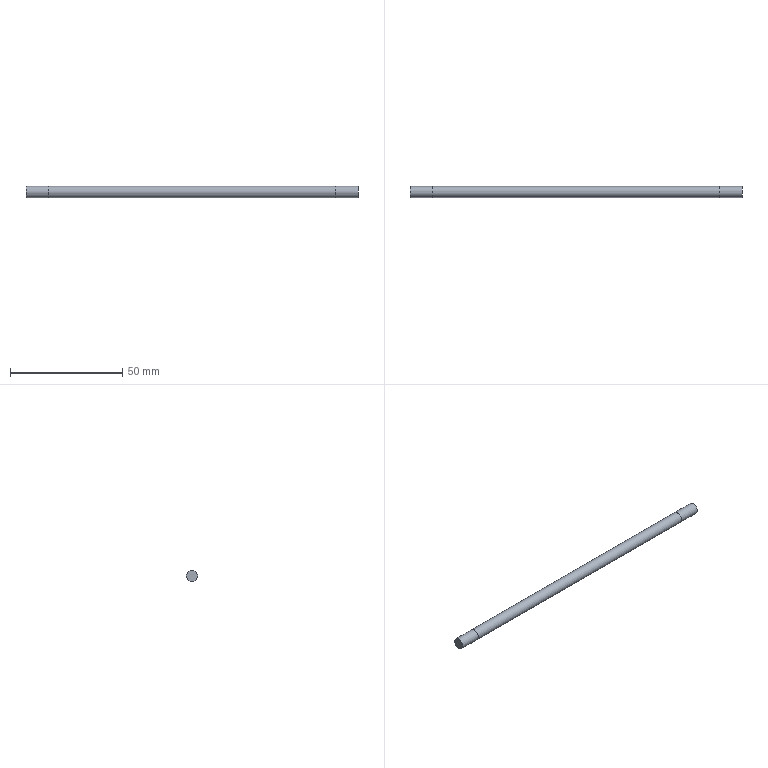Part | STEP file | 1-69.9 | 1 solid | 5 faces | box 148 x 5 x 5 mm | volume 2906 mm3 | cylinder 3 | plane 2 | commonest cylinder face diameters 5 x3
STEP:
#1=CARTESIAN_POINT('',(0.,0.,0.));
#2=DIRECTION('',(0.,0.,1.));
#3=DIRECTION('',(1.,0.,0.));
#4=AXIS2_PLACEMENT_3D('',#1,#2,#3);
#5=CARTESIAN_POINT('',(74.,2.5,0.));
#6=VERTEX_POINT('',#5);
#7=CARTESIAN_POINT('',(74.,0.,0.));
#8=DIRECTION('',(1.,0.,0.));
#9=DIRECTION('',(0.,1.,0.));
#10=AXIS2_PLACEMENT_3D('',#7,#8,#9);
#11=CIRCLE('',#10,2.5);
#12=CARTESIAN_POINT('',(74.,-0.6699,0.));
#13=DIRECTION('',(1.,0.,0.));
#14=DIRECTION('',(0.,1.,0.));
#15=AXIS2_PLACEMENT_3D('',#12,#13,#14);
#16=PLANE('',#15);
#17=CARTESIAN_POINT('',(0.6699,0.));
#18=DIRECTION('',(1.,0.));
#19=AXIS2_PLACEMENT_2D('',#17,#18);
#20=CIRCLE('',#19,2.5);
#21=(GEOMETRIC_REPRESENTATION_CONTEXT(2)PARAMETRIC_REPRESENTATION_CONTEXT()REPRESENTATION_CONTEXT('',''));
#22=DEFINITIONAL_REPRESENTATION('',(#20),#21);
#23=PCURVE('',#16,#22);
#24=CARTESIAN_POINT('',(74.,0.,0.));
#25=DIRECTION('',(-1.,0.,0.));
#26=DIRECTION('',(0.,1.,0.));
#27=AXIS2_PLACEMENT_3D('',#24,#25,#26);
#28=CYLINDRICAL_SURFACE('',#27,2.5);
#29=CARTESIAN_POINT('',(6.283,0.));
#30=DIRECTION('',(-1.,0.));
#31=VECTOR('',#30,1.);
#32=LINE('',#29,#31);
#33=(GEOMETRIC_REPRESENTATION_CONTEXT(2)PARAMETRIC_REPRESENTATION_CONTEXT()REPRESENTATION_CONTEXT('',''));
#34=DEFINITIONAL_REPRESENTATION('',(#32),#33);
#35=PCURVE('',#28,#34);
#36=SURFACE_CURVE('',#11,(#23,#35),.PCURVE_S1.);
#37=EDGE_CURVE('',#6,#6,#36,.T.);
#38=ORIENTED_EDGE('',*,*,#37,.T.);
#39=EDGE_LOOP('',(#38));
#40=FACE_BOUND('',#39,.T.);
#41=ADVANCED_FACE('',(#40),#16,.T.);
#42=CARTESIAN_POINT('',(-74.,2.5,0.));
#43=VERTEX_POINT('',#42);
#44=CARTESIAN_POINT('',(-74.,0.,0.));
#45=DIRECTION('',(1.,0.,0.));
#46=DIRECTION('',(0.,1.,0.));
#47=AXIS2_PLACEMENT_3D('',#44,#45,#46);
#48=CIRCLE('',#47,2.5);
#49=CARTESIAN_POINT('',(-74.,-0.6699,0.));
#50=DIRECTION('',(1.,0.,0.));
#51=DIRECTION('',(0.,1.,0.));
#52=AXIS2_PLACEMENT_3D('',#49,#50,#51);
#53=PLANE('',#52);
#54=CARTESIAN_POINT('',(0.6699,0.));
#55=DIRECTION('',(1.,0.));
#56=AXIS2_PLACEMENT_2D('',#54,#55);
#57=CIRCLE('',#56,2.5);
#58=(GEOMETRIC_REPRESENTATION_CONTEXT(2)PARAMETRIC_REPRESENTATION_CONTEXT()REPRESENTATION_CONTEXT('',''));
#59=DEFINITIONAL_REPRESENTATION('',(#57),#58);
#60=PCURVE('',#53,#59);
#61=CARTESIAN_POINT('',(-64.,0.,0.));
#62=DIRECTION('',(-1.,0.,0.));
#63=DIRECTION('',(0.,1.,0.));
#64=AXIS2_PLACEMENT_3D('',#61,#62,#63);
#65=CYLINDRICAL_SURFACE('',#64,2.5);
#66=CARTESIAN_POINT('',(6.283,10.));
#67=DIRECTION('',(-1.,0.));
#68=VECTOR('',#67,1.);
#69=LINE('',#66,#68);
#70=(GEOMETRIC_REPRESENTATION_CONTEXT(2)PARAMETRIC_REPRESENTATION_CONTEXT()REPRESENTATION_CONTEXT('',''));
#71=DEFINITIONAL_REPRESENTATION('',(#69),#70);
#72=PCURVE('',#65,#71);
#73=SURFACE_CURVE('',#48,(#60,#72),.PCURVE_S1.);
#74=EDGE_CURVE('',#43,#43,#73,.T.);
#75=ORIENTED_EDGE('',*,*,#74,.T.);
#76=EDGE_LOOP('',(#75));
#77=FACE_BOUND('',#76,.F.);
#78=ADVANCED_FACE('',(#77),#53,.F.);
#79=CARTESIAN_POINT('',(64.,2.5,0.));
#80=VERTEX_POINT('',#79);
#81=CARTESIAN_POINT('',(74.,2.5,0.));
#82=DIRECTION('',(-1.,0.,0.));
#83=VECTOR('',#82,1.);
#84=LINE('',#81,#83);
#85=CARTESIAN_POINT('',(6.283,0.));
#86=DIRECTION('',(0.,1.));
#87=VECTOR('',#86,1.);
#88=LINE('',#85,#87);
#89=(GEOMETRIC_REPRESENTATION_CONTEXT(2)PARAMETRIC_REPRESENTATION_CONTEXT()REPRESENTATION_CONTEXT('',''));
#90=DEFINITIONAL_REPRESENTATION('',(#88),#89);
#91=PCURVE('',#28,#90);
#92=CARTESIAN_POINT('',(0.,0.));
#93=DIRECTION('',(0.,1.));
#94=VECTOR('',#93,1.);
#95=LINE('',#92,#94);
#96=(GEOMETRIC_REPRESENTATION_CONTEXT(2)PARAMETRIC_REPRESENTATION_CONTEXT()REPRESENTATION_CONTEXT('',''));
#97=DEFINITIONAL_REPRESENTATION('',(#95),#96);
#98=PCURVE('',#28,#97);
#99=SEAM_CURVE('',#84,(#91,#98),.PCURVE_S1.);
#100=EDGE_CURVE('',#6,#80,#99,.T.);
#101=ORIENTED_EDGE('',*,*,#100,.T.);
#102=CARTESIAN_POINT('',(64.,0.,0.));
#103=DIRECTION('',(1.,0.,0.));
#104=DIRECTION('',(0.,1.,0.));
#105=AXIS2_PLACEMENT_3D('',#102,#103,#104);
#106=CIRCLE('',#105,2.5);
#107=CARTESIAN_POINT('',(6.283,10.));
#108=DIRECTION('',(-1.,0.));
#109=VECTOR('',#108,1.);
#110=LINE('',#107,#109);
#111=(GEOMETRIC_REPRESENTATION_CONTEXT(2)PARAMETRIC_REPRESENTATION_CONTEXT()REPRESENTATION_CONTEXT('',''));
#112=DEFINITIONAL_REPRESENTATION('',(#110),#111);
#113=PCURVE('',#28,#112);
#114=CARTESIAN_POINT('',(74.,0.,0.));
#115=DIRECTION('',(-1.,0.,0.));
#116=DIRECTION('',(0.,1.,0.));
#117=AXIS2_PLACEMENT_3D('',#114,#115,#116);
#118=CYLINDRICAL_SURFACE('',#117,2.5);
#119=CARTESIAN_POINT('',(6.283,10.));
#120=DIRECTION('',(-1.,0.));
#121=VECTOR('',#120,1.);
#122=LINE('',#119,#121);
#123=(GEOMETRIC_REPRESENTATION_CONTEXT(2)PARAMETRIC_REPRESENTATION_CONTEXT()REPRESENTATION_CONTEXT('',''));
#124=DEFINITIONAL_REPRESENTATION('',(#122),#123);
#125=PCURVE('',#118,#124);
#126=SURFACE_CURVE('',#106,(#113,#125),.PCURVE_S1.);
#127=EDGE_CURVE('',#80,#80,#126,.T.);
#128=ORIENTED_EDGE('',*,*,#127,.T.);
#129=ORIENTED_EDGE('',*,*,#100,.F.);
#130=ORIENTED_EDGE('',*,*,#37,.F.);
#131=EDGE_LOOP('',(#101,#128,#129,#130));
#132=FACE_BOUND('',#131,.T.);
#133=ADVANCED_FACE('',(#132),#28,.T.);
#134=CARTESIAN_POINT('',(-64.,2.5,0.));
#135=VERTEX_POINT('',#134);
#136=CARTESIAN_POINT('',(64.,2.5,0.));
#137=DIRECTION('',(-1.,0.,0.));
#138=VECTOR('',#137,1.);
#139=LINE('',#136,#138);
#140=CARTESIAN_POINT('',(6.283,10.));
#141=DIRECTION('',(0.,1.));
#142=VECTOR('',#141,1.);
#143=LINE('',#140,#142);
#144=(GEOMETRIC_REPRESENTATION_CONTEXT(2)PARAMETRIC_REPRESENTATION_CONTEXT()REPRESENTATION_CONTEXT('',''));
#145=DEFINITIONAL_REPRESENTATION('',(#143),#144);
#146=PCURVE('',#118,#145);
#147=CARTESIAN_POINT('',(0.,10.));
#148=DIRECTION('',(0.,1.));
#149=VECTOR('',#148,1.);
#150=LINE('',#147,#149);
#151=(GEOMETRIC_REPRESENTATION_CONTEXT(2)PARAMETRIC_REPRESENTATION_CONTEXT()REPRESENTATION_CONTEXT('',''));
#152=DEFINITIONAL_REPRESENTATION('',(#150),#151);
#153=PCURVE('',#118,#152);
#154=SEAM_CURVE('',#139,(#146,#153),.PCURVE_S1.);
#155=EDGE_CURVE('',#80,#135,#154,.T.);
#156=ORIENTED_EDGE('',*,*,#155,.T.);
#157=CARTESIAN_POINT('',(-64.,0.,0.));
#158=DIRECTION('',(1.,0.,0.));
#159=DIRECTION('',(0.,1.,0.));
#160=AXIS2_PLACEMENT_3D('',#157,#158,#159);
#161=CIRCLE('',#160,2.5);
#162=CARTESIAN_POINT('',(6.283,138.));
#163=DIRECTION('',(-1.,0.));
#164=VECTOR('',#163,1.);
#165=LINE('',#162,#164);
#166=(GEOMETRIC_REPRESENTATION_CONTEXT(2)PARAMETRIC_REPRESENTATION_CONTEXT()REPRESENTATION_CONTEXT('',''));
#167=DEFINITIONAL_REPRESENTATION('',(#165),#166);
#168=PCURVE('',#118,#167);
#169=CARTESIAN_POINT('',(6.283,0.));
#170=DIRECTION('',(-1.,0.));
#171=VECTOR('',#170,1.);
#172=LINE('',#169,#171);
#173=(GEOMETRIC_REPRESENTATION_CONTEXT(2)PARAMETRIC_REPRESENTATION_CONTEXT()REPRESENTATION_CONTEXT('',''));
#174=DEFINITIONAL_REPRESENTATION('',(#172),#173);
#175=PCURVE('',#65,#174);
#176=SURFACE_CURVE('',#161,(#168,#175),.PCURVE_S1.);
#177=EDGE_CURVE('',#135,#135,#176,.T.);
#178=ORIENTED_EDGE('',*,*,#177,.T.);
#179=ORIENTED_EDGE('',*,*,#155,.F.);
#180=ORIENTED_EDGE('',*,*,#127,.F.);
#181=EDGE_LOOP('',(#156,#178,#179,#180));
#182=FACE_BOUND('',#181,.T.);
#183=ADVANCED_FACE('',(#182),#118,.T.);
#184=CARTESIAN_POINT('',(-64.,2.5,0.));
#185=DIRECTION('',(-1.,0.,0.));
#186=VECTOR('',#185,1.);
#187=LINE('',#184,#186);
#188=CARTESIAN_POINT('',(0.,0.));
#189=DIRECTION('',(0.,1.));
#190=VECTOR('',#189,1.);
#191=LINE('',#188,#190);
#192=(GEOMETRIC_REPRESENTATION_CONTEXT(2)PARAMETRIC_REPRESENTATION_CONTEXT()REPRESENTATION_CONTEXT('',''));
#193=DEFINITIONAL_REPRESENTATION('',(#191),#192);
#194=PCURVE('',#65,#193);
#195=CARTESIAN_POINT('',(6.283,0.));
#196=DIRECTION('',(0.,1.));
#197=VECTOR('',#196,1.);
#198=LINE('',#195,#197);
#199=(GEOMETRIC_REPRESENTATION_CONTEXT(2)PARAMETRIC_REPRESENTATION_CONTEXT()REPRESENTATION_CONTEXT('',''));
#200=DEFINITIONAL_REPRESENTATION('',(#198),#199);
#201=PCURVE('',#65,#200);
#202=SEAM_CURVE('',#187,(#194,#201),.PCURVE_S1.);
#203=EDGE_CURVE('',#135,#43,#202,.T.);
#204=ORIENTED_EDGE('',*,*,#203,.F.);
#205=ORIENTED_EDGE('',*,*,#177,.F.);
#206=ORIENTED_EDGE('',*,*,#203,.T.);
#207=ORIENTED_EDGE('',*,*,#74,.T.);
#208=EDGE_LOOP('',(#204,#205,#206,#207));
#209=FACE_BOUND('',#208,.T.);
#210=ADVANCED_FACE('',(#209),#65,.T.);
#211=CLOSED_SHELL('',(#41,#78,#133,#183,#210));
#212=MANIFOLD_SOLID_BREP('',#211);
#213=(LENGTH_UNIT()NAMED_UNIT(*)SI_UNIT(.MILLI.,.METRE.));
#214=UNCERTAINTY_MEASURE_WITH_UNIT(LENGTH_MEASURE(0.0000001),#213,'','');
#215=(NAMED_UNIT(*)PLANE_ANGLE_UNIT()SI_UNIT($,.RADIAN.));
#216=(NAMED_UNIT(*)SI_UNIT($,.STERADIAN.)SOLID_ANGLE_UNIT());
#217=(GEOMETRIC_REPRESENTATION_CONTEXT(3)GLOBAL_UNCERTAINTY_ASSIGNED_CONTEXT((#214))GLOBAL_UNIT_ASSIGNED_CONTEXT((#213,#215,#216))REPRESENTATION_CONTEXT('',''));
#218=ADVANCED_BREP_SHAPE_REPRESENTATION('',(#4,#212),#217);